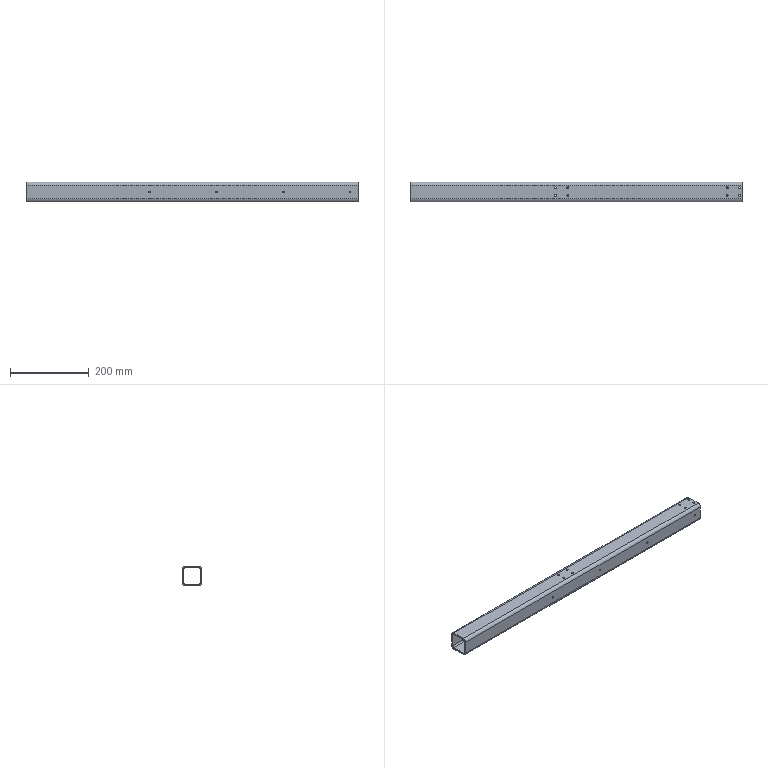Part | SolidWorks | features HoleWzd 2, ICE 1, WeldMemberFeat 1, WeldmentFeature 1 | 1 solid | 58 faces | box 845 x 50 x 50 mm | volume 585625 mm3 | cylinder 48 | plane 10 | commonest cylinder face diameters 5 x32 4.2 x8 8 x4 16 x4